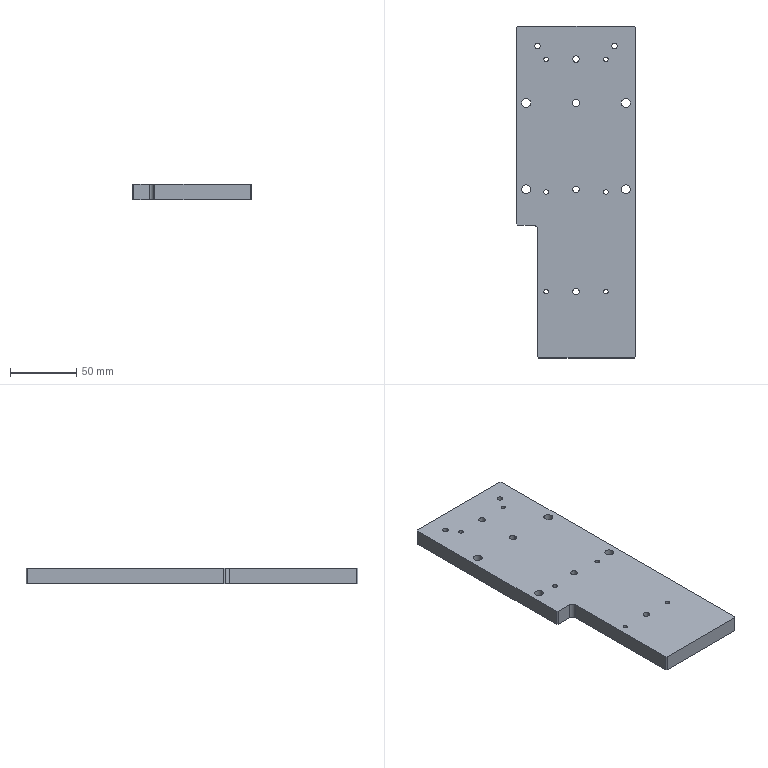CAM job | NX | 3-axis milling, drilling | part box 90 x 250 x 12 mm | stock box 100 x 255 x 15 mm
Tools:
number,name,description,diameter,corner_radius,flute_length,length,flutes
4,D4,平底铣刀-粗,4.0,0.0,25.0,75.0,2
6,D6,平底铣刀-粗,6.0,0.0,25.0,75.0,2
9,D10,平底铣刀-粗,10.0,0.0,35.0,75.0,2
11,D4-J,平底铣刀-精,4.0,0.0,50.0,75.0,2
7,D6-J,平底铣刀-精,6.0,0.0,25.0,75.0,2
1,D80R0.8_FLYCUTTER,圆鼻刀-粗,80.0,0.8,50.0,75.0,2
1,D80R0.8_FLYCUTTER-J,圆鼻刀-精,80.0,0.8,50.0,75.0,2
2,D6_CHAMFER,倒角刀,6.0,0.0,3.0,25.0,2
21,M4X0.7,丝锥,3.3,0.0,35.0,50.0,2
22,M5X0.8,丝锥,4.2,0.0,35.0,50.0,2
19,D5_REAMER,Drilling Tool,5.0,0.0,75.0,100.0,6
13,ZT3.4,钻头,3.4,0.0,35.0,50.0,2
18,6.6_DRILL,Drilling Tool,6.6,0.0,35.0,50.0,2
17,ZT4.9,Drilling Tool,4.9,0.0,35.0,50.0,2
14,ZT4.3,Drilling Tool,4.3,0.0,50.0,75.0,4
Operations:
program,operation,operation_type,tool,method,geometry_group,spindle_rpm,surface_speed,feed_per_tooth,feed_cut,feed_plunge,cut_length_mm,path_length_mm,cut_time_min,machine_time_min
A,TOPFACE,FaceMilling,D80R0.8_FLYCUTTER,SIDEFINISH-DEPTHK-STEPG,W-A,4500.0,1385.0,0.1667,1500.0,100.0,1089.0,1185.0,0.726,0.7356
A,DYNROUGHD10_COPY,CavityMilling,D10,DYNROUGH-DEPTHK-STEPK,W-A,8000.0,251.32,0.25,4000.0,100.0,8235.912,8661.365,2.059,2.102
A,SPOT-DEPTH0.8,Operation,D6_CHAMFER,NONE,W-A,8000.0,150.796,0.0312,500.0,90.0,27.0,588.728,0.054,0.1102
A,SPOT-DEPTH0.8_COPY,Operation,D6_CHAMFER,NONE,W-A,8000.0,150.796,0.0312,500.0,90.0,1.8,103.6,0.0036,0.0138
A,THRUHOLE-M4TAPDRILL,Operation,ZT3.4,NONE,W-A,3000.0,31.102,0.05,300.0,90.0,114.0,643.045,0.38,0.4329
A,THRUHOLE-M5TAPDRILL,Operation,ZT4.3,NONE,W-A,3000.0,39.584,0.0583,350.0,90.0,40.0,239.009,0.1143,0.1342
A,THRUHOLE-6.0PREDRILL,Operation,ZT4.9,NONE,W-A,2500.0,38.484,0.05,250.0,90.0,52.243,381.499,0.209,0.2419
A,THRUHOLE-6.0PREDRILL_COPY,Operation,ZT4.9,NONE,W-A,2500.0,38.484,0.05,250.0,90.0,17.415,134.829,0.0697,0.0814
A,COUNTERBORE-DRILLSEG0,Operation,6.6_DRILL,NONE,W-A,1200.0,24.881,0.0625,150.0,90.0,67.621,443.264,0.4508,0.4884
A,KIDNEYSLOTROUGH_1,VolumeBased25DMillingOperation,D4,METHOD,W-A,12000.0,150.796,0.0208,500.0,100.0,416.856,527.556,0.8337,0.8448
A,HOLEROUGHD6_1,CylinderMilling,D6,NONE,W-A,8000.0,150.796,0.075,1200.0,100.0,923.332,1551.932,0.7694,0.8323
A,HOLEFINISHD6_1,CylinderMilling,D6-J,FINISHSTEPDEPTHOFF,W-A,8000.0,150.796,0.0312,500.0,100.0,178.461,809.061,0.3569,0.42
A,ZLEVELSMOOTHCORNERD6REF12_COPY,ZLevelMilling,D6-J,LAYERFINISH-DEPTHK-STEPG,W-A,8000.0,150.796,0.1375,2200.0,100.0,523.059,634.109,0.2378,0.2489
A,SELECTBODYONLY,SurfaceContour,D6_CHAMFER,METHOD,W-A,8000.0,150.796,0.1875,3000.0,100.0,711.768,985.093,0.2373,0.2646
A,NG_DRILLCHAMFER_1,Operation,D6_CHAMFER,METHOD,W-A,8000.0,150.796,0.0312,500.0,0.0,31.2,487.805,0.0624,0.1081
A,MILLCHAMFER_1,PlanarMilling,D6_CHAMFER,METHOD,W-A,8000.0,150.796,0.0312,500.0,100.0,36.041,296.057,0.0721,0.0981
A,MILLCHAMFER_2,PlanarMilling,D6_CHAMFER,METHOD,W-A,8000.0,150.796,0.0312,500.0,100.0,55.445,536.582,0.1109,0.159
A,MILLCHAMFER_3,PlanarMilling,D6_CHAMFER,NONE,W-A,8000.0,150.796,0.05,800.0,100.0,173.57,756.67,0.217,0.2753
A,THRUHOLE-TAPM4,Operation,M4X0.7,METHOD,W-A,600.0,6.22,0.0006,0.7,90.0,96.0,607.045,137.143,137.194
A,THRUHOLE-TAPM5,Operation,M5X0.8,METHOD,W-A,500.0,6.597,0.0008,0.8,90.0,33.0,225.009,41.25,41.269
A,REAM,Operation,D5_REAMER,METHOD,W-A,500.0,7.854,0.0167,50.0,0.0,42.0,361.012,0.84,0.8719
A,KIDNEYSLOTFINISH_1,VolumeBased25DMillingOperation,D4-J,METHOD,W-A,8000.0,100.531,0.0125,200.0,100.0,22.518,163.324,0.1126,0.1267
A,PROFILESEMIFINISH_2,VolumeBased25DMillingOperation,D6-J,METHOD,W-A,9000.0,169.646,0.0667,1200.0,100.0,699.549,822.549,0.583,0.5953
B,FLOORFLYROUGH_COPY,VolumeBased25DMillingOperation,D80R0.8_FLYCUTTER,LAYERROUGH-DEPTHK-STEPG,W-B,2800.0,703.696,0.5357,3000.0,100.0,3583.487,3816.714,1.194,1.218
B,FLOORFLYFINISH_COPY,VolumeBased25DMillingOperation,D80R0.8_FLYCUTTER-J,SIDEFINISH-DEPTHK-STEPG,W-B,4000.0,1005.28,0.125,1000.0,100.0,716.11,812.11,0.7161,0.7257
B,NG_DRILLCHAMFER_2,Operation,D6_CHAMFER,METHOD,W-B,8000.0,150.796,0.0625,1000.0,0.0,31.2,487.805,0.0312,0.0769
B,NG_DRILLCHAMFER_3,Operation,D6_CHAMFER,METHOD,W-B,8000.0,150.796,0.0625,1000.0,0.0,11.4,183.877,0.0114,0.0286
B,NG_DRILLCHAMFER_DJ10_1,Operation,D6_CHAMFER,METHOD,W-B,8000.0,150.796,0.0625,1000.0,0.0,17.4,315.904,0.0174,0.0473
B,MILLCHAMFER_4,PlanarMilling,D6_CHAMFER,METHOD,W-B,8000.0,150.796,0.075,1200.0,100.0,81.784,694.015,0.0682,0.1294
B,PLANARDEBURR6X45L_COPY,SurfaceContour,D6_CHAMFER,CLIMBFACE_CHAMFER-DEPTH0-STEPG,W-B,6500.0,122.519,0.1154,1500.0,100.0,884.659,1831.838,0.5898,0.6845